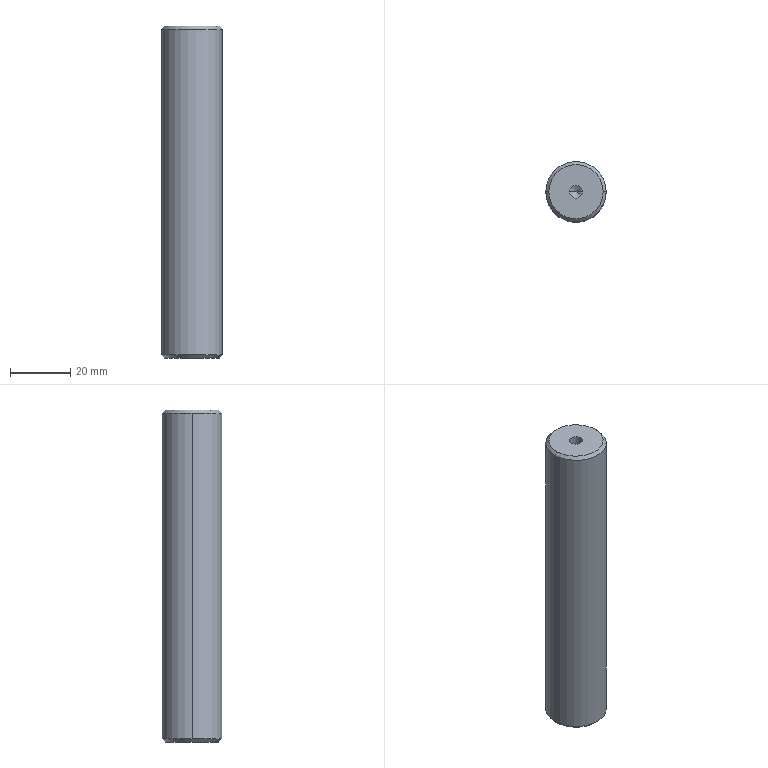Part | STEP file | 1 solid | 16 faces | box 20 x 20 x 110 mm | volume 33959 mm3 | cone 8 | cylinder 6 | plane 2 | commonest cylinder face diameters 4.2 x4 20 x2
STEP:
#1=CARTESIAN_POINT('',(0.,0.,0.));
#2=DIRECTION('',(0.,0.,1.));
#3=DIRECTION('',(1.,0.,0.));
#4=AXIS2_PLACEMENT_3D('',#1,#2,#3);
#5=CARTESIAN_POINT('',(9.,0.,110.));
#6=VERTEX_POINT('',#5);
#7=CARTESIAN_POINT('',(-9.,0.,110.));
#8=VERTEX_POINT('',#7);
#9=CARTESIAN_POINT('',(0.,0.,110.));
#10=DIRECTION('',(0.,0.,1.));
#11=DIRECTION('',(1.,0.,0.));
#12=AXIS2_PLACEMENT_3D('',#9,#10,#11);
#13=CIRCLE('',#12,9.);
#14=CARTESIAN_POINT('',(0.,0.,110.));
#15=DIRECTION('',(0.,0.,-1.));
#16=DIRECTION('',(-1.,0.,0.));
#17=AXIS2_PLACEMENT_3D('',#14,#15,#16);
#18=CONICAL_SURFACE('',#17,9.,0.7854);
#19=CARTESIAN_POINT('',(3.142,0.));
#20=DIRECTION('',(-1.,0.));
#21=VECTOR('',#20,1.);
#22=LINE('',#19,#21);
#23=(GEOMETRIC_REPRESENTATION_CONTEXT(2)PARAMETRIC_REPRESENTATION_CONTEXT()REPRESENTATION_CONTEXT('',''));
#24=DEFINITIONAL_REPRESENTATION('',(#22),#23);
#25=PCURVE('',#18,#24);
#26=CARTESIAN_POINT('',(0.,0.,110.));
#27=DIRECTION('',(0.,0.,1.));
#28=DIRECTION('',(1.,0.,0.));
#29=AXIS2_PLACEMENT_3D('',#26,#27,#28);
#30=PLANE('',#29);
#31=CARTESIAN_POINT('',(0.,0.));
#32=DIRECTION('',(1.,0.));
#33=AXIS2_PLACEMENT_2D('',#31,#32);
#34=CIRCLE('',#33,9.);
#35=(GEOMETRIC_REPRESENTATION_CONTEXT(2)PARAMETRIC_REPRESENTATION_CONTEXT()REPRESENTATION_CONTEXT('',''));
#36=DEFINITIONAL_REPRESENTATION('',(#34),#35);
#37=PCURVE('',#30,#36);
#38=SURFACE_CURVE('',#13,(#25,#37),.PCURVE_S1.);
#39=EDGE_CURVE('',#6,#8,#38,.T.);
#40=ORIENTED_EDGE('',*,*,#39,.F.);
#41=CARTESIAN_POINT('',(10.,0.,109.));
#42=VERTEX_POINT('',#41);
#43=CARTESIAN_POINT('',(9.,0.,110.));
#44=DIRECTION('',(0.7071,0.,-0.7071));
#45=VECTOR('',#44,1.);
#46=LINE('',#43,#45);
#47=CARTESIAN_POINT('',(3.142,0.));
#48=DIRECTION('',(0.,1.));
#49=VECTOR('',#48,1.);
#50=LINE('',#47,#49);
#51=(GEOMETRIC_REPRESENTATION_CONTEXT(2)PARAMETRIC_REPRESENTATION_CONTEXT()REPRESENTATION_CONTEXT('',''));
#52=DEFINITIONAL_REPRESENTATION('',(#50),#51);
#53=PCURVE('',#18,#52);
#54=CARTESIAN_POINT('',(0.,0.,110.));
#55=DIRECTION('',(0.,0.,-1.));
#56=DIRECTION('',(-1.,0.,0.));
#57=AXIS2_PLACEMENT_3D('',#54,#55,#56);
#58=CONICAL_SURFACE('',#57,9.,0.7854);
#59=CARTESIAN_POINT('',(3.142,0.));
#60=DIRECTION('',(0.,1.));
#61=VECTOR('',#60,1.);
#62=LINE('',#59,#61);
#63=(GEOMETRIC_REPRESENTATION_CONTEXT(2)PARAMETRIC_REPRESENTATION_CONTEXT()REPRESENTATION_CONTEXT('',''));
#64=DEFINITIONAL_REPRESENTATION('',(#62),#63);
#65=PCURVE('',#58,#64);
#66=SURFACE_CURVE('',#46,(#53,#65),.PCURVE_S1.);
#67=EDGE_CURVE('',#6,#42,#66,.T.);
#68=ORIENTED_EDGE('',*,*,#67,.T.);
#69=CARTESIAN_POINT('',(-10.,0.,109.));
#70=VERTEX_POINT('',#69);
#71=CARTESIAN_POINT('',(0.,0.,109.));
#72=DIRECTION('',(0.,0.,-1.));
#73=DIRECTION('',(1.,0.,0.));
#74=AXIS2_PLACEMENT_3D('',#71,#72,#73);
#75=CIRCLE('',#74,10.);
#76=CARTESIAN_POINT('',(-3.142,1.));
#77=DIRECTION('',(1.,0.));
#78=VECTOR('',#77,1.);
#79=LINE('',#76,#78);
#80=(GEOMETRIC_REPRESENTATION_CONTEXT(2)PARAMETRIC_REPRESENTATION_CONTEXT()REPRESENTATION_CONTEXT('',''));
#81=DEFINITIONAL_REPRESENTATION('',(#79),#80);
#82=PCURVE('',#18,#81);
#83=CARTESIAN_POINT('',(0.,0.,110.));
#84=DIRECTION('',(0.,0.,-1.));
#85=DIRECTION('',(-1.,0.,0.));
#86=AXIS2_PLACEMENT_3D('',#83,#84,#85);
#87=CYLINDRICAL_SURFACE('',#86,10.);
#88=CARTESIAN_POINT('',(-3.142,1.));
#89=DIRECTION('',(1.,0.));
#90=VECTOR('',#89,1.);
#91=LINE('',#88,#90);
#92=(GEOMETRIC_REPRESENTATION_CONTEXT(2)PARAMETRIC_REPRESENTATION_CONTEXT()REPRESENTATION_CONTEXT('',''));
#93=DEFINITIONAL_REPRESENTATION('',(#91),#92);
#94=PCURVE('',#87,#93);
#95=SURFACE_CURVE('',#75,(#82,#94),.PCURVE_S1.);
#96=EDGE_CURVE('',#70,#42,#95,.T.);
#97=ORIENTED_EDGE('',*,*,#96,.F.);
#98=CARTESIAN_POINT('',(-9.,0.,110.));
#99=DIRECTION('',(-0.7071,0.,-0.7071));
#100=VECTOR('',#99,1.);
#101=LINE('',#98,#100);
#102=CARTESIAN_POINT('',(0.,0.));
#103=DIRECTION('',(0.,1.));
#104=VECTOR('',#103,1.);
#105=LINE('',#102,#104);
#106=(GEOMETRIC_REPRESENTATION_CONTEXT(2)PARAMETRIC_REPRESENTATION_CONTEXT()REPRESENTATION_CONTEXT('',''));
#107=DEFINITIONAL_REPRESENTATION('',(#105),#106);
#108=PCURVE('',#18,#107);
#109=CARTESIAN_POINT('',(6.283,0.));
#110=DIRECTION('',(0.,1.));
#111=VECTOR('',#110,1.);
#112=LINE('',#109,#111);
#113=(GEOMETRIC_REPRESENTATION_CONTEXT(2)PARAMETRIC_REPRESENTATION_CONTEXT()REPRESENTATION_CONTEXT('',''));
#114=DEFINITIONAL_REPRESENTATION('',(#112),#113);
#115=PCURVE('',#58,#114);
#116=SURFACE_CURVE('',#101,(#108,#115),.PCURVE_S1.);
#117=EDGE_CURVE('',#8,#70,#116,.T.);
#118=ORIENTED_EDGE('',*,*,#117,.F.);
#119=EDGE_LOOP('',(#40,#68,#97,#118));
#120=FACE_BOUND('',#119,.T.);
#121=ADVANCED_FACE('',(#120),#18,.T.);
#122=CARTESIAN_POINT('',(-9.,0.,0.));
#123=VERTEX_POINT('',#122);
#124=CARTESIAN_POINT('',(9.,0.,0.));
#125=VERTEX_POINT('',#124);
#126=CARTESIAN_POINT('',(0.,0.,0.));
#127=DIRECTION('',(0.,0.,-1.));
#128=DIRECTION('',(1.,0.,0.));
#129=AXIS2_PLACEMENT_3D('',#126,#127,#128);
#130=CIRCLE('',#129,9.);
#131=CARTESIAN_POINT('',(0.,0.,1.));
#132=DIRECTION('',(0.,0.,1.));
#133=DIRECTION('',(1.,0.,0.));
#134=AXIS2_PLACEMENT_3D('',#131,#132,#133);
#135=CONICAL_SURFACE('',#134,10.,0.7854);
#136=CARTESIAN_POINT('',(6.283,-1.));
#137=DIRECTION('',(-1.,0.));
#138=VECTOR('',#137,1.);
#139=LINE('',#136,#138);
#140=(GEOMETRIC_REPRESENTATION_CONTEXT(2)PARAMETRIC_REPRESENTATION_CONTEXT()REPRESENTATION_CONTEXT('',''));
#141=DEFINITIONAL_REPRESENTATION('',(#139),#140);
#142=PCURVE('',#135,#141);
#143=CARTESIAN_POINT('',(0.,0.,0.));
#144=DIRECTION('',(0.,0.,1.));
#145=DIRECTION('',(1.,0.,0.));
#146=AXIS2_PLACEMENT_3D('',#143,#144,#145);
#147=PLANE('',#146);
#148=CARTESIAN_POINT('',(9.,0.));
#149=CARTESIAN_POINT('',(9.,-15.588));
#150=CARTESIAN_POINT('',(-4.5,-7.794));
#151=CARTESIAN_POINT('',(-18.,0.));
#152=CARTESIAN_POINT('',(-4.5,7.794));
#153=CARTESIAN_POINT('',(9.,15.588));
#154=CARTESIAN_POINT('',(9.,0.));
#155=(BOUNDED_CURVE()B_SPLINE_CURVE(2,(#148,#149,#150,#151,#152,#153,#154),.UNSPECIFIED.,.T.,.F.)B_SPLINE_CURVE_WITH_KNOTS((1,2,2,2,2,1),(-2.094,0.,2.094,4.189,6.283,8.378),.UNSPECIFIED.)CURVE()GEOMETRIC_REPRESENTATION_ITEM()RATIONAL_B_SPLINE_CURVE((1.,0.5,1.,0.5,1.,0.5,1.))REPRESENTATION_ITEM(''));
#156=(GEOMETRIC_REPRESENTATION_CONTEXT(2)PARAMETRIC_REPRESENTATION_CONTEXT()REPRESENTATION_CONTEXT('',''));
#157=DEFINITIONAL_REPRESENTATION('',(#155),#156);
#158=PCURVE('',#147,#157);
#159=SURFACE_CURVE('',#130,(#142,#158),.PCURVE_S1.);
#160=EDGE_CURVE('',#123,#125,#159,.T.);
#161=ORIENTED_EDGE('',*,*,#160,.F.);
#162=CARTESIAN_POINT('',(-10.,0.,1.));
#163=VERTEX_POINT('',#162);
#164=CARTESIAN_POINT('',(-10.,0.,1.));
#165=DIRECTION('',(-0.7071,0.,0.7071));
#166=VECTOR('',#165,1.);
#167=LINE('',#164,#166);
#168=CARTESIAN_POINT('',(3.142,0.));
#169=DIRECTION('',(0.,1.));
#170=VECTOR('',#169,1.);
#171=LINE('',#168,#170);
#172=(GEOMETRIC_REPRESENTATION_CONTEXT(2)PARAMETRIC_REPRESENTATION_CONTEXT()REPRESENTATION_CONTEXT('',''));
#173=DEFINITIONAL_REPRESENTATION('',(#171),#172);
#174=PCURVE('',#135,#173);
#175=CARTESIAN_POINT('',(0.,0.,1.));
#176=DIRECTION('',(0.,0.,1.));
#177=DIRECTION('',(1.,0.,0.));
#178=AXIS2_PLACEMENT_3D('',#175,#176,#177);
#179=CONICAL_SURFACE('',#178,10.,0.7854);
#180=CARTESIAN_POINT('',(3.142,0.));
#181=DIRECTION('',(0.,1.));
#182=VECTOR('',#181,1.);
#183=LINE('',#180,#182);
#184=(GEOMETRIC_REPRESENTATION_CONTEXT(2)PARAMETRIC_REPRESENTATION_CONTEXT()REPRESENTATION_CONTEXT('',''));
#185=DEFINITIONAL_REPRESENTATION('',(#183),#184);
#186=PCURVE('',#179,#185);
#187=SURFACE_CURVE('',#167,(#174,#186),.PCURVE_S1.);
#188=EDGE_CURVE('',#123,#163,#187,.T.);
#189=ORIENTED_EDGE('',*,*,#188,.T.);
#190=CARTESIAN_POINT('',(10.,0.,1.));
#191=VERTEX_POINT('',#190);
#192=CARTESIAN_POINT('',(0.,0.,1.));
#193=DIRECTION('',(0.,0.,1.));
#194=DIRECTION('',(1.,0.,0.));
#195=AXIS2_PLACEMENT_3D('',#192,#193,#194);
#196=CIRCLE('',#195,10.);
#197=CARTESIAN_POINT('',(0.,0.));
#198=DIRECTION('',(1.,0.));
#199=VECTOR('',#198,1.);
#200=LINE('',#197,#199);
#201=(GEOMETRIC_REPRESENTATION_CONTEXT(2)PARAMETRIC_REPRESENTATION_CONTEXT()REPRESENTATION_CONTEXT('',''));
#202=DEFINITIONAL_REPRESENTATION('',(#200),#201);
#203=PCURVE('',#135,#202);
#204=CARTESIAN_POINT('',(3.142,109.));
#205=DIRECTION('',(-1.,0.));
#206=VECTOR('',#205,1.);
#207=LINE('',#204,#206);
#208=(GEOMETRIC_REPRESENTATION_CONTEXT(2)PARAMETRIC_REPRESENTATION_CONTEXT()REPRESENTATION_CONTEXT('',''));
#209=DEFINITIONAL_REPRESENTATION('',(#207),#208);
#210=PCURVE('',#87,#209);
#211=SURFACE_CURVE('',#196,(#203,#210),.PCURVE_S1.);
#212=EDGE_CURVE('',#191,#163,#211,.T.);
#213=ORIENTED_EDGE('',*,*,#212,.F.);
#214=CARTESIAN_POINT('',(10.,0.,1.));
#215=DIRECTION('',(0.7071,0.,0.7071));
#216=VECTOR('',#215,1.);
#217=LINE('',#214,#216);
#218=CARTESIAN_POINT('',(0.,0.));
#219=DIRECTION('',(0.,1.));
#220=VECTOR('',#219,1.);
#221=LINE('',#218,#220);
#222=(GEOMETRIC_REPRESENTATION_CONTEXT(2)PARAMETRIC_REPRESENTATION_CONTEXT()REPRESENTATION_CONTEXT('',''));
#223=DEFINITIONAL_REPRESENTATION('',(#221),#222);
#224=PCURVE('',#135,#223);
#225=CARTESIAN_POINT('',(6.283,0.));
#226=DIRECTION('',(0.,1.));
#227=VECTOR('',#226,1.);
#228=LINE('',#225,#227);
#229=(GEOMETRIC_REPRESENTATION_CONTEXT(2)PARAMETRIC_REPRESENTATION_CONTEXT()REPRESENTATION_CONTEXT('',''));
#230=DEFINITIONAL_REPRESENTATION('',(#228),#229);
#231=PCURVE('',#179,#230);
#232=SURFACE_CURVE('',#217,(#224,#231),.PCURVE_S1.);
#233=EDGE_CURVE('',#125,#191,#232,.T.);
#234=ORIENTED_EDGE('',*,*,#233,.F.);
#235=EDGE_LOOP('',(#161,#189,#213,#234));
#236=FACE_BOUND('',#235,.T.);
#237=ADVANCED_FACE('',(#236),#135,.T.);
#238=CARTESIAN_POINT('',(2.1,0.,91.));
#239=VERTEX_POINT('',#238);
#240=CARTESIAN_POINT('',(2.1,0.,110.));
#241=VERTEX_POINT('',#240);
#242=CARTESIAN_POINT('',(2.1,0.,110.));
#243=DIRECTION('',(0.,0.,1.));
#244=VECTOR('',#243,1.);
#245=LINE('',#242,#244);
#246=CARTESIAN_POINT('',(0.,0.,110.));
#247=DIRECTION('',(0.,0.,1.));
#248=DIRECTION('',(1.,0.,0.));
#249=AXIS2_PLACEMENT_3D('',#246,#247,#248);
#250=CYLINDRICAL_SURFACE('',#249,2.1);
#251=CARTESIAN_POINT('',(6.283,0.));
#252=DIRECTION('',(0.,1.));
#253=VECTOR('',#252,1.);
#254=LINE('',#251,#253);
#255=(GEOMETRIC_REPRESENTATION_CONTEXT(2)PARAMETRIC_REPRESENTATION_CONTEXT()REPRESENTATION_CONTEXT('',''));
#256=DEFINITIONAL_REPRESENTATION('',(#254),#255);
#257=PCURVE('',#250,#256);
#258=CARTESIAN_POINT('',(0.,0.,110.));
#259=DIRECTION('',(0.,0.,1.));
#260=DIRECTION('',(1.,0.,0.));
#261=AXIS2_PLACEMENT_3D('',#258,#259,#260);
#262=CYLINDRICAL_SURFACE('',#261,2.1);
#263=CARTESIAN_POINT('',(0.,0.));
#264=DIRECTION('',(0.,1.));
#265=VECTOR('',#264,1.);
#266=LINE('',#263,#265);
#267=(GEOMETRIC_REPRESENTATION_CONTEXT(2)PARAMETRIC_REPRESENTATION_CONTEXT()REPRESENTATION_CONTEXT('',''));
#268=DEFINITIONAL_REPRESENTATION('',(#266),#267);
#269=PCURVE('',#262,#268);
#270=SURFACE_CURVE('',#245,(#257,#269),.PCURVE_S1.);
#271=EDGE_CURVE('',#239,#241,#270,.T.);
#272=ORIENTED_EDGE('',*,*,#271,.T.);
#273=CARTESIAN_POINT('',(-2.1,0.,110.));
#274=VERTEX_POINT('',#273);
#275=CARTESIAN_POINT('',(0.,0.,110.));
#276=DIRECTION('',(0.,0.,1.));
#277=DIRECTION('',(1.,0.,0.));
#278=AXIS2_PLACEMENT_3D('',#275,#276,#277);
#279=CIRCLE('',#278,2.1);
#280=CARTESIAN_POINT('',(0.,0.));
#281=DIRECTION('',(1.,0.));
#282=VECTOR('',#281,1.);
#283=LINE('',#280,#282);
#284=(GEOMETRIC_REPRESENTATION_CONTEXT(2)PARAMETRIC_REPRESENTATION_CONTEXT()REPRESENTATION_CONTEXT('',''));
#285=DEFINITIONAL_REPRESENTATION('',(#283),#284);
#286=PCURVE('',#250,#285);
#287=CARTESIAN_POINT('',(0.,0.));
#288=DIRECTION('',(1.,0.));
#289=AXIS2_PLACEMENT_2D('',#287,#288);
#290=CIRCLE('',#289,2.1);
#291=(GEOMETRIC_REPRESENTATION_CONTEXT(2)PARAMETRIC_REPRESENTATION_CONTEXT()REPRESENTATION_CONTEXT('',''));
#292=DEFINITIONAL_REPRESENTATION('',(#290),#291);
#293=PCURVE('',#30,#292);
#294=SURFACE_CURVE('',#279,(#286,#293),.PCURVE_S1.);
#295=EDGE_CURVE('',#274,#241,#294,.T.);
#296=ORIENTED_EDGE('',*,*,#295,.F.);
#297=CARTESIAN_POINT('',(-2.1,0.,91.));
#298=VERTEX_POINT('',#297);
#299=CARTESIAN_POINT('',(-2.1,0.,110.));
#300=DIRECTION('',(0.,0.,1.));
#301=VECTOR('',#300,1.);
#302=LINE('',#299,#301);
#303=CARTESIAN_POINT('',(3.142,0.));
#304=DIRECTION('',(0.,1.));
#305=VECTOR('',#304,1.);
#306=LINE('',#303,#305);
#307=(GEOMETRIC_REPRESENTATION_CONTEXT(2)PARAMETRIC_REPRESENTATION_CONTEXT()REPRESENTATION_CONTEXT('',''));
#308=DEFINITIONAL_REPRESENTATION('',(#306),#307);
#309=PCURVE('',#250,#308);
#310=CARTESIAN_POINT('',(3.142,0.));
#311=DIRECTION('',(0.,1.));
#312=VECTOR('',#311,1.);
#313=LINE('',#310,#312);
#314=(GEOMETRIC_REPRESENTATION_CONTEXT(2)PARAMETRIC_REPRESENTATION_CONTEXT()REPRESENTATION_CONTEXT('',''));
#315=DEFINITIONAL_REPRESENTATION('',(#313),#314);
#316=PCURVE('',#262,#315);
#317=SURFACE_CURVE('',#302,(#309,#316),.PCURVE_S1.);
#318=EDGE_CURVE('',#298,#274,#317,.T.);
#319=ORIENTED_EDGE('',*,*,#318,.F.);
#320=CARTESIAN_POINT('',(0.,0.,91.));
#321=DIRECTION('',(0.,0.,1.));
#322=DIRECTION('',(1.,0.,0.));
#323=AXIS2_PLACEMENT_3D('',#320,#321,#322);
#324=CIRCLE('',#323,2.1);
#325=CARTESIAN_POINT('',(0.,-19.));
#326=DIRECTION('',(1.,0.));
#327=VECTOR('',#326,1.);
#328=LINE('',#325,#327);
#329=(GEOMETRIC_REPRESENTATION_CONTEXT(2)PARAMETRIC_REPRESENTATION_CONTEXT()REPRESENTATION_CONTEXT('',''));
#330=DEFINITIONAL_REPRESENTATION('',(#328),#329);
#331=PCURVE('',#250,#330);
#332=CARTESIAN_POINT('',(0.,0.,91.));
#333=DIRECTION('',(0.,0.,1.));
#334=DIRECTION('',(1.,0.,0.));
#335=AXIS2_PLACEMENT_3D('',#332,#333,#334);
#336=CONICAL_SURFACE('',#335,2.1,1.03);
#337=CARTESIAN_POINT('',(0.,0.));
#338=DIRECTION('',(1.,0.));
#339=VECTOR('',#338,1.);
#340=LINE('',#337,#339);
#341=(GEOMETRIC_REPRESENTATION_CONTEXT(2)PARAMETRIC_REPRESENTATION_CONTEXT()REPRESENTATION_CONTEXT('',''));
#342=DEFINITIONAL_REPRESENTATION('',(#340),#341);
#343=PCURVE('',#336,#342);
#344=SURFACE_CURVE('',#324,(#331,#343),.PCURVE_S1.);
#345=EDGE_CURVE('',#298,#239,#344,.T.);
#346=ORIENTED_EDGE('',*,*,#345,.T.);
#347=EDGE_LOOP('',(#272,#296,#319,#346));
#348=FACE_BOUND('',#347,.F.);
#349=ADVANCED_FACE('',(#348),#250,.F.);
#350=ORIENTED_EDGE('',*,*,#345,.F.);
#351=CARTESIAN_POINT('',(0.,0.,89.738));
#352=VERTEX_POINT('',#351);
#353=CARTESIAN_POINT('',(-2.1,0.,91.));
#354=DIRECTION('',(-0.8572,0.,0.515));
#355=VECTOR('',#354,1.);
#356=LINE('',#353,#355);
#357=CARTESIAN_POINT('',(3.142,0.));
#358=DIRECTION('',(0.,1.));
#359=VECTOR('',#358,1.);
#360=LINE('',#357,#359);
#361=(GEOMETRIC_REPRESENTATION_CONTEXT(2)PARAMETRIC_REPRESENTATION_CONTEXT()REPRESENTATION_CONTEXT('',''));
#362=DEFINITIONAL_REPRESENTATION('',(#360),#361);
#363=PCURVE('',#336,#362);
#364=CARTESIAN_POINT('',(0.,0.,91.));
#365=DIRECTION('',(0.,0.,1.));
#366=DIRECTION('',(1.,0.,0.));
#367=AXIS2_PLACEMENT_3D('',#364,#365,#366);
#368=CONICAL_SURFACE('',#367,2.1,1.03);
#369=CARTESIAN_POINT('',(3.142,0.));
#370=DIRECTION('',(0.,1.));
#371=VECTOR('',#370,1.);
#372=LINE('',#369,#371);
#373=(GEOMETRIC_REPRESENTATION_CONTEXT(2)PARAMETRIC_REPRESENTATION_CONTEXT()REPRESENTATION_CONTEXT('',''));
#374=DEFINITIONAL_REPRESENTATION('',(#372),#373);
#375=PCURVE('',#368,#374);
#376=SURFACE_CURVE('',#356,(#363,#375),.PCURVE_S1.);
#377=EDGE_CURVE('',#352,#298,#376,.T.);
#378=ORIENTED_EDGE('',*,*,#377,.F.);
#379=CARTESIAN_POINT('',(2.1,0.,91.));
#380=DIRECTION('',(0.8572,0.,0.515));
#381=VECTOR('',#380,1.);
#382=LINE('',#379,#381);
#383=CARTESIAN_POINT('',(6.283,-1.262));
#384=CARTESIAN_POINT('',(6.283,-1.243));
#385=CARTESIAN_POINT('',(6.283,-1.204));
#386=CARTESIAN_POINT('',(6.283,-1.147));
#387=CARTESIAN_POINT('',(6.283,-1.09));
#388=CARTESIAN_POINT('',(6.283,-1.032));
#389=CARTESIAN_POINT('',(6.283,-0.975));
#390=CARTESIAN_POINT('',(6.283,-0.9177));
#391=CARTESIAN_POINT('',(6.283,-0.8603));
#392=CARTESIAN_POINT('',(6.283,-0.803));
#393=CARTESIAN_POINT('',(6.283,-0.7456));
#394=CARTESIAN_POINT('',(6.283,-0.6883));
#395=CARTESIAN_POINT('',(6.283,-0.6309));
#396=CARTESIAN_POINT('',(6.283,-0.5735));
#397=CARTESIAN_POINT('',(6.283,-0.5162));
#398=CARTESIAN_POINT('',(6.283,-0.4588));
#399=CARTESIAN_POINT('',(6.283,-0.4015));
#400=CARTESIAN_POINT('',(6.283,-0.3441));
#401=CARTESIAN_POINT('',(6.283,-0.2868));
#402=CARTESIAN_POINT('',(6.283,-0.2294));
#403=CARTESIAN_POINT('',(6.283,-0.1721));
#404=CARTESIAN_POINT('',(6.283,-0.1147));
#405=CARTESIAN_POINT('',(6.283,-0.05735));
#406=CARTESIAN_POINT('',(6.283,-0.01912));
#407=CARTESIAN_POINT('',(6.283,0.));
#408=B_SPLINE_CURVE_WITH_KNOTS('',3,(#383,#384,#385,#386,#387,#388,#389,#390,#391,#392,#393,#394,#395,#396,#397,#398,#399,#400,#401,#402,#403,#404,#405,#406,#407),.UNSPECIFIED.,.F.,.F.,(4,1,1,1,1,1,1,1,1,1,1,1,1,1,1,1,1,1,1,1,1,1,4),(-2.45,-2.339,-2.227,-2.116,-2.004,-1.893,-1.782,-1.67,-1.559,-1.448,-1.336,-1.225,-1.114,-1.002,-0.8909,-0.7795,-0.6682,-0.5568,-0.4454,-0.3341,-0.2227,-0.1114,0.),.QUASI_UNIFORM_KNOTS.);
#409=(GEOMETRIC_REPRESENTATION_CONTEXT(2)PARAMETRIC_REPRESENTATION_CONTEXT()REPRESENTATION_CONTEXT('',''));
#410=DEFINITIONAL_REPRESENTATION('',(#408),#409);
#411=PCURVE('',#336,#410);
#412=CARTESIAN_POINT('',(0.,-1.262));
#413=CARTESIAN_POINT('',(0.,-1.243));
#414=CARTESIAN_POINT('',(0.,-1.204));
#415=CARTESIAN_POINT('',(0.,-1.147));
#416=CARTESIAN_POINT('',(0.,-1.09));
#417=CARTESIAN_POINT('',(0.,-1.032));
#418=CARTESIAN_POINT('',(0.,-0.975));
#419=CARTESIAN_POINT('',(0.,-0.9177));
#420=CARTESIAN_POINT('',(0.,-0.8603));
#421=CARTESIAN_POINT('',(0.,-0.803));
#422=CARTESIAN_POINT('',(0.,-0.7456));
#423=CARTESIAN_POINT('',(0.,-0.6883));
#424=CARTESIAN_POINT('',(0.,-0.6309));
#425=CARTESIAN_POINT('',(0.,-0.5735));
#426=CARTESIAN_POINT('',(0.,-0.5162));
#427=CARTESIAN_POINT('',(0.,-0.4588));
#428=CARTESIAN_POINT('',(0.,-0.4015));
#429=CARTESIAN_POINT('',(0.,-0.3441));
#430=CARTESIAN_POINT('',(0.,-0.2868));
#431=CARTESIAN_POINT('',(0.,-0.2294));
#432=CARTESIAN_POINT('',(0.,-0.1721));
#433=CARTESIAN_POINT('',(0.,-0.1147));
#434=CARTESIAN_POINT('',(0.,-0.05735));
#435=CARTESIAN_POINT('',(0.,-0.01912));
#436=CARTESIAN_POINT('',(0.,0.));
#437=B_SPLINE_CURVE_WITH_KNOTS('',3,(#412,#413,#414,#415,#416,#417,#418,#419,#420,#421,#422,#423,#424,#425,#426,#427,#428,#429,#430,#431,#432,#433,#434,#435,#436),.UNSPECIFIED.,.F.,.F.,(4,1,1,1,1,1,1,1,1,1,1,1,1,1,1,1,1,1,1,1,1,1,4),(-2.45,-2.339,-2.227,-2.116,-2.004,-1.893,-1.782,-1.67,-1.559,-1.448,-1.336,-1.225,-1.114,-1.002,-0.8909,-0.7795,-0.6682,-0.5568,-0.4454,-0.3341,-0.2227,-0.1114,0.),.QUASI_UNIFORM_KNOTS.);
#438=(GEOMETRIC_REPRESENTATION_CONTEXT(2)PARAMETRIC_REPRESENTATION_CONTEXT()REPRESENTATION_CONTEXT('',''));
#439=DEFINITIONAL_REPRESENTATION('',(#437),#438);
#440=PCURVE('',#368,#439);
#441=SURFACE_CURVE('',#382,(#411,#440),.PCURVE_S1.);
#442=EDGE_CURVE('',#352,#239,#441,.T.);
#443=ORIENTED_EDGE('',*,*,#442,.T.);
#444=EDGE_LOOP('',(#350,#378,#443));
#445=FACE_BOUND('',#444,.F.);
#446=ADVANCED_FACE('',(#445),#336,.F.);
#447=CARTESIAN_POINT('',(-2.1,0.,19.));
#448=VERTEX_POINT('',#447);
#449=CARTESIAN_POINT('',(-2.1,0.,0.));
#450=VERTEX_POINT('',#449);
#451=CARTESIAN_POINT('',(-2.1,0.,0.));
#452=DIRECTION('',(0.,0.,-1.));
#453=VECTOR('',#452,1.);
#454=LINE('',#451,#453);
#455=CARTESIAN_POINT('',(0.,0.,0.));
#456=DIRECTION('',(0.,0.,-1.));
#457=DIRECTION('',(-1.,0.,0.));
#458=AXIS2_PLACEMENT_3D('',#455,#456,#457);
#459=CYLINDRICAL_SURFACE('',#458,2.1);
#460=CARTESIAN_POINT('',(6.283,0.));
#461=DIRECTION('',(0.,1.));
#462=VECTOR('',#461,1.);
#463=LINE('',#460,#462);
#464=(GEOMETRIC_REPRESENTATION_CONTEXT(2)PARAMETRIC_REPRESENTATION_CONTEXT()REPRESENTATION_CONTEXT('',''));
#465=DEFINITIONAL_REPRESENTATION('',(#463),#464);
#466=PCURVE('',#459,#465);
#467=CARTESIAN_POINT('',(0.,0.,0.));
#468=DIRECTION('',(0.,0.,-1.));
#469=DIRECTION('',(-1.,0.,0.));
#470=AXIS2_PLACEMENT_3D('',#467,#468,#469);
#471=CYLINDRICAL_SURFACE('',#470,2.1);
#472=CARTESIAN_POINT('',(0.,0.));
#473=DIRECTION('',(0.,1.));
#474=VECTOR('',#473,1.);
#475=LINE('',#472,#474);
#476=(GEOMETRIC_REPRESENTATION_CONTEXT(2)PARAMETRIC_REPRESENTATION_CONTEXT()REPRESENTATION_CONTEXT('',''));
#477=DEFINITIONAL_REPRESENTATION('',(#475),#476);
#478=PCURVE('',#471,#477);
#479=SURFACE_CURVE('',#454,(#466,#478),.PCURVE_S1.);
#480=EDGE_CURVE('',#448,#450,#479,.T.);
#481=ORIENTED_EDGE('',*,*,#480,.T.);
#482=CARTESIAN_POINT('',(2.1,0.,0.));
#483=VERTEX_POINT('',#482);
#484=CARTESIAN_POINT('',(0.,0.,0.));
#485=DIRECTION('',(0.,0.,-1.));
#486=DIRECTION('',(-1.,0.,0.));
#487=AXIS2_PLACEMENT_3D('',#484,#485,#486);
#488=CIRCLE('',#487,2.1);
#489=CARTESIAN_POINT('',(0.,0.));
#490=DIRECTION('',(1.,0.));
#491=VECTOR('',#490,1.);
#492=LINE('',#489,#491);
#493=(GEOMETRIC_REPRESENTATION_CONTEXT(2)PARAMETRIC_REPRESENTATION_CONTEXT()REPRESENTATION_CONTEXT('',''));
#494=DEFINITIONAL_REPRESENTATION('',(#492),#493);
#495=PCURVE('',#459,#494);
#496=CARTESIAN_POINT('',(-2.1,0.));
#497=CARTESIAN_POINT('',(-2.1,3.637));
#498=CARTESIAN_POINT('',(1.05,1.819));
#499=CARTESIAN_POINT('',(4.2,0.));
#500=CARTESIAN_POINT('',(1.05,-1.819));
#501=CARTESIAN_POINT('',(-2.1,-3.637));
#502=CARTESIAN_POINT('',(-2.1,0.));
#503=(BOUNDED_CURVE()B_SPLINE_CURVE(2,(#496,#497,#498,#499,#500,#501,#502),.UNSPECIFIED.,.T.,.F.)B_SPLINE_CURVE_WITH_KNOTS((1,2,2,2,2,1),(-2.094,0.,2.094,4.189,6.283,8.378),.UNSPECIFIED.)CURVE()GEOMETRIC_REPRESENTATION_ITEM()RATIONAL_B_SPLINE_CURVE((1.,0.5,1.,0.5,1.,0.5,1.))REPRESENTATION_ITEM(''));
#504=(GEOMETRIC_REPRESENTATION_CONTEXT(2)PARAMETRIC_REPRESENTATION_CONTEXT()REPRESENTATION_CONTEXT('',''));
#505=DEFINITIONAL_REPRESENTATION('',(#503),#504);
#506=PCURVE('',#147,#505);
#507=SURFACE_CURVE('',#488,(#495,#506),.PCURVE_S1.);
#508=EDGE_CURVE('',#483,#450,#507,.T.);
#509=ORIENTED_EDGE('',*,*,#508,.F.);
#510=CARTESIAN_POINT('',(2.1,0.,19.));
#511=VERTEX_POINT('',#510);
#512=CARTESIAN_POINT('',(2.1,0.,0.));
#513=DIRECTION('',(0.,0.,-1.));
#514=VECTOR('',#513,1.);
#515=LINE('',#512,#514);
#516=CARTESIAN_POINT('',(3.142,0.));
#517=DIRECTION('',(0.,1.));
#518=VECTOR('',#517,1.);
#519=LINE('',#516,#518);
#520=(GEOMETRIC_REPRESENTATION_CONTEXT(2)PARAMETRIC_REPRESENTATION_CONTEXT()REPRESENTATION_CONTEXT('',''));
#521=DEFINITIONAL_REPRESENTATION('',(#519),#520);
#522=PCURVE('',#459,#521);
#523=CARTESIAN_POINT('',(3.142,0.));
#524=DIRECTION('',(0.,1.));
#525=VECTOR('',#524,1.);
#526=LINE('',#523,#525);
#527=(GEOMETRIC_REPRESENTATION_CONTEXT(2)PARAMETRIC_REPRESENTATION_CONTEXT()REPRESENTATION_CONTEXT('',''));
#528=DEFINITIONAL_REPRESENTATION('',(#526),#527);
#529=PCURVE('',#471,#528);
#530=SURFACE_CURVE('',#515,(#522,#529),.PCURVE_S1.);
#531=EDGE_CURVE('',#511,#483,#530,.T.);
#532=ORIENTED_EDGE('',*,*,#531,.F.);
#533=CARTESIAN_POINT('',(0.,0.,19.));
#534=DIRECTION('',(0.,0.,-1.));
#535=DIRECTION('',(-1.,0.,0.));
#536=AXIS2_PLACEMENT_3D('',#533,#534,#535);
#537=CIRCLE('',#536,2.1);
#538=CARTESIAN_POINT('',(0.,-19.));
#539=DIRECTION('',(1.,0.));
#540=VECTOR('',#539,1.);
#541=LINE('',#538,#540);
#542=(GEOMETRIC_REPRESENTATION_CONTEXT(2)PARAMETRIC_REPRESENTATION_CONTEXT()REPRESENTATION_CONTEXT('',''));
#543=DEFINITIONAL_REPRESENTATION('',(#541),#542);
#544=PCURVE('',#459,#543);
#545=CARTESIAN_POINT('',(0.,0.,19.));
#546=DIRECTION('',(0.,0.,-1.));
#547=DIRECTION('',(-1.,0.,0.));
#548=AXIS2_PLACEMENT_3D('',#545,#546,#547);
#549=CONICAL_SURFACE('',#548,2.1,1.03);
#550=CARTESIAN_POINT('',(0.,0.));
#551=DIRECTION('',(1.,0.));
#552=VECTOR('',#551,1.);
#553=LINE('',#550,#552);
#554=(GEOMETRIC_REPRESENTATION_CONTEXT(2)PARAMETRIC_REPRESENTATION_CONTEXT()REPRESENTATION_CONTEXT('',''));
#555=DEFINITIONAL_REPRESENTATION('',(#553),#554);
#556=PCURVE('',#549,#555);
#557=SURFACE_CURVE('',#537,(#544,#556),.PCURVE_S1.);
#558=EDGE_CURVE('',#511,#448,#557,.T.);
#559=ORIENTED_EDGE('',*,*,#558,.T.);
#560=EDGE_LOOP('',(#481,#509,#532,#559));
#561=FACE_BOUND('',#560,.F.);
#562=ADVANCED_FACE('',(#561),#459,.F.);
#563=ORIENTED_EDGE('',*,*,#558,.F.);
#564=CARTESIAN_POINT('',(0.,0.,20.262));
#565=VERTEX_POINT('',#564);
#566=CARTESIAN_POINT('',(2.1,0.,19.));
#567=DIRECTION('',(0.8572,0.,-0.515));
#568=VECTOR('',#567,1.);
#569=LINE('',#566,#568);
#570=CARTESIAN_POINT('',(3.142,-1.262));
#571=CARTESIAN_POINT('',(3.142,-1.243));
#572=CARTESIAN_POINT('',(3.142,-1.204));
#573=CARTESIAN_POINT('',(3.142,-1.147));
#574=CARTESIAN_POINT('',(3.142,-1.09));
#575=CARTESIAN_POINT('',(3.142,-1.032));
#576=CARTESIAN_POINT('',(3.142,-0.975));
#577=CARTESIAN_POINT('',(3.142,-0.9177));
#578=CARTESIAN_POINT('',(3.142,-0.8603));
#579=CARTESIAN_POINT('',(3.142,-0.803));
#580=CARTESIAN_POINT('',(3.142,-0.7456));
#581=CARTESIAN_POINT('',(3.142,-0.6883));
#582=CARTESIAN_POINT('',(3.142,-0.6309));
#583=CARTESIAN_POINT('',(3.142,-0.5735));
#584=CARTESIAN_POINT('',(3.142,-0.5162));
#585=CARTESIAN_POINT('',(3.142,-0.4588));
#586=CARTESIAN_POINT('',(3.142,-0.4015));
#587=CARTESIAN_POINT('',(3.142,-0.3441));
#588=CARTESIAN_POINT('',(3.142,-0.2868));
#589=CARTESIAN_POINT('',(3.142,-0.2294));
#590=CARTESIAN_POINT('',(3.142,-0.1721));
#591=CARTESIAN_POINT('',(3.142,-0.1147));
#592=CARTESIAN_POINT('',(3.142,-0.05735));
#593=CARTESIAN_POINT('',(3.142,-0.01912));
#594=CARTESIAN_POINT('',(3.142,0.));
#595=B_SPLINE_CURVE_WITH_KNOTS('',3,(#570,#571,#572,#573,#574,#575,#576,#577,#578,#579,#580,#581,#582,#583,#584,#585,#586,#587,#588,#589,#590,#591,#592,#593,#594),.UNSPECIFIED.,.F.,.F.,(4,1,1,1,1,1,1,1,1,1,1,1,1,1,1,1,1,1,1,1,1,1,4),(-2.45,-2.339,-2.227,-2.116,-2.004,-1.893,-1.782,-1.67,-1.559,-1.448,-1.336,-1.225,-1.114,-1.002,-0.8909,-0.7795,-0.6682,-0.5568,-0.4454,-0.3341,-0.2227,-0.1114,0.),.UNSPECIFIED.);
#596=(GEOMETRIC_REPRESENTATION_CONTEXT(2)PARAMETRIC_REPRESENTATION_CONTEXT()REPRESENTATION_CONTEXT('',''));
#597=DEFINITIONAL_REPRESENTATION('',(#595),#596);
#598=PCURVE('',#549,#597);
#599=CARTESIAN_POINT('',(0.,0.,19.));
#600=DIRECTION('',(0.,0.,-1.));
#601=DIRECTION('',(-1.,0.,0.));
#602=AXIS2_PLACEMENT_3D('',#599,#600,#601);
#603=CONICAL_SURFACE('',#602,2.1,1.03);
#604=CARTESIAN_POINT('',(3.142,-1.262));
#605=CARTESIAN_POINT('',(3.142,-1.243));
#606=CARTESIAN_POINT('',(3.142,-1.204));
#607=CARTESIAN_POINT('',(3.142,-1.147));
#608=CARTESIAN_POINT('',(3.142,-1.09));
#609=CARTESIAN_POINT('',(3.142,-1.032));
#610=CARTESIAN_POINT('',(3.142,-0.975));
#611=CARTESIAN_POINT('',(3.142,-0.9177));
#612=CARTESIAN_POINT('',(3.142,-0.8603));
#613=CARTESIAN_POINT('',(3.142,-0.803));
#614=CARTESIAN_POINT('',(3.142,-0.7456));
#615=CARTESIAN_POINT('',(3.142,-0.6883));
#616=CARTESIAN_POINT('',(3.142,-0.6309));
#617=CARTESIAN_POINT('',(3.142,-0.5735));
#618=CARTESIAN_POINT('',(3.142,-0.5162));
#619=CARTESIAN_POINT('',(3.142,-0.4588));
#620=CARTESIAN_POINT('',(3.142,-0.4015));
#621=CARTESIAN_POINT('',(3.142,-0.3441));
#622=CARTESIAN_POINT('',(3.142,-0.2868));
#623=CARTESIAN_POINT('',(3.142,-0.2294));
#624=CARTESIAN_POINT('',(3.142,-0.1721));
#625=CARTESIAN_POINT('',(3.142,-0.1147));
#626=CARTESIAN_POINT('',(3.142,-0.05735));
#627=CARTESIAN_POINT('',(3.142,-0.01912));
#628=CARTESIAN_POINT('',(3.142,0.));
#629=B_SPLINE_CURVE_WITH_KNOTS('',3,(#604,#605,#606,#607,#608,#609,#610,#611,#612,#613,#614,#615,#616,#617,#618,#619,#620,#621,#622,#623,#624,#625,#626,#627,#628),.UNSPECIFIED.,.F.,.F.,(4,1,1,1,1,1,1,1,1,1,1,1,1,1,1,1,1,1,1,1,1,1,4),(-2.45,-2.339,-2.227,-2.116,-2.004,-1.893,-1.782,-1.67,-1.559,-1.448,-1.336,-1.225,-1.114,-1.002,-0.8909,-0.7795,-0.6682,-0.5568,-0.4454,-0.3341,-0.2227,-0.1114,0.),.UNSPECIFIED.);
#630=(GEOMETRIC_REPRESENTATION_CONTEXT(2)PARAMETRIC_REPRESENTATION_CONTEXT()REPRESENTATION_CONTEXT('',''));
#631=DEFINITIONAL_REPRESENTATION('',(#629),#630);
#632=PCURVE('',#603,#631);
#633=SURFACE_CURVE('',#569,(#598,#632),.PCURVE_S1.);
#634=EDGE_CURVE('',#565,#511,#633,.T.);
#635=ORIENTED_EDGE('',*,*,#634,.F.);
#636=CARTESIAN_POINT('',(-2.1,0.,19.));
#637=DIRECTION('',(-0.8572,0.,-0.515));
#638=VECTOR('',#637,1.);
#639=LINE('',#636,#638);
#640=CARTESIAN_POINT('',(6.283,0.));
#641=DIRECTION('',(0.,1.));
#642=VECTOR('',#641,1.);
#643=LINE('',#640,#642);
#644=(GEOMETRIC_REPRESENTATION_CONTEXT(2)PARAMETRIC_REPRESENTATION_CONTEXT()REPRESENTATION_CONTEXT('',''));
#645=DEFINITIONAL_REPRESENTATION('',(#643),#644);
#646=PCURVE('',#549,#645);
#647=CARTESIAN_POINT('',(0.,0.));
#648=DIRECTION('',(0.,1.));
#649=VECTOR('',#648,1.);
#650=LINE('',#647,#649);
#651=(GEOMETRIC_REPRESENTATION_CONTEXT(2)PARAMETRIC_REPRESENTATION_CONTEXT()REPRESENTATION_CONTEXT('',''));
#652=DEFINITIONAL_REPRESENTATION('',(#650),#651);
#653=PCURVE('',#603,#652);
#654=SURFACE_CURVE('',#639,(#646,#653),.PCURVE_S1.);
#655=EDGE_CURVE('',#565,#448,#654,.T.);
#656=ORIENTED_EDGE('',*,*,#655,.T.);
#657=EDGE_LOOP('',(#563,#635,#656));
#658=FACE_BOUND('',#657,.F.);
#659=ADVANCED_FACE('',(#658),#549,.F.);
#660=ORIENTED_EDGE('',*,*,#96,.T.);
#661=CARTESIAN_POINT('',(10.,0.,110.));
#662=DIRECTION('',(0.,0.,-1.));
#663=VECTOR('',#662,1.);
#664=LINE('',#661,#663);
#665=CARTESIAN_POINT('',(3.142,0.));
#666=DIRECTION('',(0.,1.));
#667=VECTOR('',#666,1.);
#668=LINE('',#665,#667);
#669=(GEOMETRIC_REPRESENTATION_CONTEXT(2)PARAMETRIC_REPRESENTATION_CONTEXT()REPRESENTATION_CONTEXT('',''));
#670=DEFINITIONAL_REPRESENTATION('',(#668),#669);
#671=PCURVE('',#87,#670);
#672=CARTESIAN_POINT('',(0.,0.,110.));
#673=DIRECTION('',(0.,0.,-1.));
#674=DIRECTION('',(-1.,0.,0.));
#675=AXIS2_PLACEMENT_3D('',#672,#673,#674);
#676=CYLINDRICAL_SURFACE('',#675,10.);
#677=CARTESIAN_POINT('',(3.142,0.));
#678=DIRECTION('',(0.,1.));
#679=VECTOR('',#678,1.);
#680=LINE('',#677,#679);
#681=(GEOMETRIC_REPRESENTATION_CONTEXT(2)PARAMETRIC_REPRESENTATION_CONTEXT()REPRESENTATION_CONTEXT('',''));
#682=DEFINITIONAL_REPRESENTATION('',(#680),#681);
#683=PCURVE('',#676,#682);
#684=SURFACE_CURVE('',#664,(#671,#683),.PCURVE_S1.);
#685=EDGE_CURVE('',#42,#191,#684,.T.);
#686=ORIENTED_EDGE('',*,*,#685,.T.);
#687=ORIENTED_EDGE('',*,*,#212,.T.);
#688=CARTESIAN_POINT('',(-10.,0.,110.));
#689=DIRECTION('',(0.,0.,-1.));
#690=VECTOR('',#689,1.);
#691=LINE('',#688,#690);
#692=CARTESIAN_POINT('',(0.,0.));
#693=DIRECTION('',(0.,1.));
#694=VECTOR('',#693,1.);
#695=LINE('',#692,#694);
#696=(GEOMETRIC_REPRESENTATION_CONTEXT(2)PARAMETRIC_REPRESENTATION_CONTEXT()REPRESENTATION_CONTEXT('',''));
#697=DEFINITIONAL_REPRESENTATION('',(#695),#696);
#698=PCURVE('',#87,#697);
#699=CARTESIAN_POINT('',(6.283,0.));
#700=DIRECTION('',(0.,1.));
#701=VECTOR('',#700,1.);
#702=LINE('',#699,#701);
#703=(GEOMETRIC_REPRESENTATION_CONTEXT(2)PARAMETRIC_REPRESENTATION_CONTEXT()REPRESENTATION_CONTEXT('',''));
#704=DEFINITIONAL_REPRESENTATION('',(#702),#703);
#705=PCURVE('',#676,#704);
#706=SURFACE_CURVE('',#691,(#698,#705),.PCURVE_S1.);
#707=EDGE_CURVE('',#70,#163,#706,.T.);
#708=ORIENTED_EDGE('',*,*,#707,.F.);
#709=EDGE_LOOP('',(#660,#686,#687,#708));
#710=FACE_BOUND('',#709,.T.);
#711=ADVANCED_FACE('',(#710),#87,.T.);
#712=ORIENTED_EDGE('',*,*,#685,.F.);
#713=CARTESIAN_POINT('',(0.,0.,109.));
#714=DIRECTION('',(0.,0.,-1.));
#715=DIRECTION('',(1.,0.,0.));
#716=AXIS2_PLACEMENT_3D('',#713,#714,#715);
#717=CIRCLE('',#716,10.);
#718=CARTESIAN_POINT('',(3.142,1.));
#719=DIRECTION('',(1.,0.));
#720=VECTOR('',#719,1.);
#721=LINE('',#718,#720);
#722=(GEOMETRIC_REPRESENTATION_CONTEXT(2)PARAMETRIC_REPRESENTATION_CONTEXT()REPRESENTATION_CONTEXT('',''));
#723=DEFINITIONAL_REPRESENTATION('',(#721),#722);
#724=PCURVE('',#676,#723);
#725=CARTESIAN_POINT('',(3.142,1.));
#726=DIRECTION('',(1.,0.));
#727=VECTOR('',#726,1.);
#728=LINE('',#725,#727);
#729=(GEOMETRIC_REPRESENTATION_CONTEXT(2)PARAMETRIC_REPRESENTATION_CONTEXT()REPRESENTATION_CONTEXT('',''));
#730=DEFINITIONAL_REPRESENTATION('',(#728),#729);
#731=PCURVE('',#58,#730);
#732=SURFACE_CURVE('',#717,(#724,#731),.PCURVE_S1.);
#733=EDGE_CURVE('',#42,#70,#732,.T.);
#734=ORIENTED_EDGE('',*,*,#733,.T.);
#735=ORIENTED_EDGE('',*,*,#707,.T.);
#736=CARTESIAN_POINT('',(0.,0.,1.));
#737=DIRECTION('',(0.,0.,1.));
#738=DIRECTION('',(1.,0.,0.));
#739=AXIS2_PLACEMENT_3D('',#736,#737,#738);
#740=CIRCLE('',#739,10.);
#741=CARTESIAN_POINT('',(9.425,109.));
#742=DIRECTION('',(-1.,0.));
#743=VECTOR('',#742,1.);
#744=LINE('',#741,#743);
#745=(GEOMETRIC_REPRESENTATION_CONTEXT(2)PARAMETRIC_REPRESENTATION_CONTEXT()REPRESENTATION_CONTEXT('',''));
#746=DEFINITIONAL_REPRESENTATION('',(#744),#745);
#747=PCURVE('',#676,#746);
#748=CARTESIAN_POINT('',(0.,0.));
#749=DIRECTION('',(1.,0.));
#750=VECTOR('',#749,1.);
#751=LINE('',#748,#750);
#752=(GEOMETRIC_REPRESENTATION_CONTEXT(2)PARAMETRIC_REPRESENTATION_CONTEXT()REPRESENTATION_CONTEXT('',''));
#753=DEFINITIONAL_REPRESENTATION('',(#751),#752);
#754=PCURVE('',#179,#753);
#755=SURFACE_CURVE('',#740,(#747,#754),.PCURVE_S1.);
#756=EDGE_CURVE('',#163,#191,#755,.T.);
#757=ORIENTED_EDGE('',*,*,#756,.T.);
#758=EDGE_LOOP('',(#712,#734,#735,#757));
#759=FACE_BOUND('',#758,.T.);
#760=ADVANCED_FACE('',(#759),#676,.T.);
#761=CARTESIAN_POINT('',(0.,0.,110.));
#762=DIRECTION('',(0.,0.,1.));
#763=DIRECTION('',(1.,0.,0.));
#764=AXIS2_PLACEMENT_3D('',#761,#762,#763);
#765=CIRCLE('',#764,9.);
#766=CARTESIAN_POINT('',(0.,0.));
#767=DIRECTION('',(1.,0.));
#768=AXIS2_PLACEMENT_2D('',#766,#767);
#769=CIRCLE('',#768,9.);
#770=(GEOMETRIC_REPRESENTATION_CONTEXT(2)PARAMETRIC_REPRESENTATION_CONTEXT()REPRESENTATION_CONTEXT('',''));
#771=DEFINITIONAL_REPRESENTATION('',(#769),#770);
#772=PCURVE('',#30,#771);
#773=CARTESIAN_POINT('',(9.425,0.));
#774=DIRECTION('',(-1.,0.));
#775=VECTOR('',#774,1.);
#776=LINE('',#773,#775);
#777=(GEOMETRIC_REPRESENTATION_CONTEXT(2)PARAMETRIC_REPRESENTATION_CONTEXT()REPRESENTATION_CONTEXT('',''));
#778=DEFINITIONAL_REPRESENTATION('',(#776),#777);
#779=PCURVE('',#58,#778);
#780=SURFACE_CURVE('',#765,(#772,#779),.PCURVE_S1.);
#781=EDGE_CURVE('',#8,#6,#780,.T.);
#782=ORIENTED_EDGE('',*,*,#781,.T.);
#783=ORIENTED_EDGE('',*,*,#39,.T.);
#784=EDGE_LOOP('',(#782,#783));
#785=FACE_BOUND('',#784,.T.);
#786=CARTESIAN_POINT('',(0.,0.,110.));
#787=DIRECTION('',(0.,0.,1.));
#788=DIRECTION('',(1.,0.,0.));
#789=AXIS2_PLACEMENT_3D('',#786,#787,#788);
#790=CIRCLE('',#789,2.1);
#791=CARTESIAN_POINT('',(0.,0.));
#792=DIRECTION('',(1.,0.));
#793=AXIS2_PLACEMENT_2D('',#791,#792);
#794=CIRCLE('',#793,2.1);
#795=(GEOMETRIC_REPRESENTATION_CONTEXT(2)PARAMETRIC_REPRESENTATION_CONTEXT()REPRESENTATION_CONTEXT('',''));
#796=DEFINITIONAL_REPRESENTATION('',(#794),#795);
#797=PCURVE('',#30,#796);
#798=CARTESIAN_POINT('',(0.,0.));
#799=DIRECTION('',(1.,0.));
#800=VECTOR('',#799,1.);
#801=LINE('',#798,#800);
#802=(GEOMETRIC_REPRESENTATION_CONTEXT(2)PARAMETRIC_REPRESENTATION_CONTEXT()REPRESENTATION_CONTEXT('',''));
#803=DEFINITIONAL_REPRESENTATION('',(#801),#802);
#804=PCURVE('',#262,#803);
#805=SURFACE_CURVE('',#790,(#797,#804),.PCURVE_S1.);
#806=EDGE_CURVE('',#241,#274,#805,.T.);
#807=ORIENTED_EDGE('',*,*,#806,.F.);
#808=ORIENTED_EDGE('',*,*,#295,.F.);
#809=EDGE_LOOP('',(#807,#808));
#810=FACE_BOUND('',#809,.T.);
#811=ADVANCED_FACE('',(#785,#810),#30,.T.);
#812=CARTESIAN_POINT('',(0.,0.,0.));
#813=DIRECTION('',(0.,0.,-1.));
#814=DIRECTION('',(1.,0.,0.));
#815=AXIS2_PLACEMENT_3D('',#812,#813,#814);
#816=CIRCLE('',#815,9.);
#817=CARTESIAN_POINT('',(9.,0.));
#818=CARTESIAN_POINT('',(9.,-15.588));
#819=CARTESIAN_POINT('',(-4.5,-7.794));
#820=CARTESIAN_POINT('',(-18.,0.));
#821=CARTESIAN_POINT('',(-4.5,7.794));
#822=CARTESIAN_POINT('',(9.,15.588));
#823=CARTESIAN_POINT('',(9.,0.));
#824=(BOUNDED_CURVE()B_SPLINE_CURVE(2,(#817,#818,#819,#820,#821,#822,#823),.UNSPECIFIED.,.T.,.F.)B_SPLINE_CURVE_WITH_KNOTS((1,2,2,2,2,1),(-2.094,0.,2.094,4.189,6.283,8.378),.UNSPECIFIED.)CURVE()GEOMETRIC_REPRESENTATION_ITEM()RATIONAL_B_SPLINE_CURVE((1.,0.5,1.,0.5,1.,0.5,1.))REPRESENTATION_ITEM(''));
#825=(GEOMETRIC_REPRESENTATION_CONTEXT(2)PARAMETRIC_REPRESENTATION_CONTEXT()REPRESENTATION_CONTEXT('',''));
#826=DEFINITIONAL_REPRESENTATION('',(#824),#825);
#827=PCURVE('',#147,#826);
#828=CARTESIAN_POINT('',(6.283,-1.));
#829=DIRECTION('',(-1.,0.));
#830=VECTOR('',#829,1.);
#831=LINE('',#828,#830);
#832=(GEOMETRIC_REPRESENTATION_CONTEXT(2)PARAMETRIC_REPRESENTATION_CONTEXT()REPRESENTATION_CONTEXT('',''));
#833=DEFINITIONAL_REPRESENTATION('',(#831),#832);
#834=PCURVE('',#179,#833);
#835=SURFACE_CURVE('',#816,(#827,#834),.PCURVE_S1.);
#836=EDGE_CURVE('',#125,#123,#835,.T.);
#837=ORIENTED_EDGE('',*,*,#836,.T.);
#838=ORIENTED_EDGE('',*,*,#160,.T.);
#839=EDGE_LOOP('',(#837,#838));
#840=FACE_BOUND('',#839,.T.);
#841=CARTESIAN_POINT('',(0.,0.,0.));
#842=DIRECTION('',(0.,0.,-1.));
#843=DIRECTION('',(-1.,0.,0.));
#844=AXIS2_PLACEMENT_3D('',#841,#842,#843);
#845=CIRCLE('',#844,2.1);
#846=CARTESIAN_POINT('',(-2.1,0.));
#847=CARTESIAN_POINT('',(-2.1,3.637));
#848=CARTESIAN_POINT('',(1.05,1.819));
#849=CARTESIAN_POINT('',(4.2,0.));
#850=CARTESIAN_POINT('',(1.05,-1.819));
#851=CARTESIAN_POINT('',(-2.1,-3.637));
#852=CARTESIAN_POINT('',(-2.1,0.));
#853=(BOUNDED_CURVE()B_SPLINE_CURVE(2,(#846,#847,#848,#849,#850,#851,#852),.UNSPECIFIED.,.T.,.F.)B_SPLINE_CURVE_WITH_KNOTS((1,2,2,2,2,1),(-2.094,0.,2.094,4.189,6.283,8.378),.UNSPECIFIED.)CURVE()GEOMETRIC_REPRESENTATION_ITEM()RATIONAL_B_SPLINE_CURVE((1.,0.5,1.,0.5,1.,0.5,1.))REPRESENTATION_ITEM(''));
#854=(GEOMETRIC_REPRESENTATION_CONTEXT(2)PARAMETRIC_REPRESENTATION_CONTEXT()REPRESENTATION_CONTEXT('',''));
#855=DEFINITIONAL_REPRESENTATION('',(#853),#854);
#856=PCURVE('',#147,#855);
#857=CARTESIAN_POINT('',(0.,0.));
#858=DIRECTION('',(1.,0.));
#859=VECTOR('',#858,1.);
#860=LINE('',#857,#859);
#861=(GEOMETRIC_REPRESENTATION_CONTEXT(2)PARAMETRIC_REPRESENTATION_CONTEXT()REPRESENTATION_CONTEXT('',''));
#862=DEFINITIONAL_REPRESENTATION('',(#860),#861);
#863=PCURVE('',#471,#862);
#864=SURFACE_CURVE('',#845,(#856,#863),.PCURVE_S1.);
#865=EDGE_CURVE('',#450,#483,#864,.T.);
#866=ORIENTED_EDGE('',*,*,#865,.F.);
#867=ORIENTED_EDGE('',*,*,#508,.F.);
#868=EDGE_LOOP('',(#866,#867));
#869=FACE_BOUND('',#868,.T.);
#870=ADVANCED_FACE('',(#840,#869),#147,.F.);
#871=CARTESIAN_POINT('',(0.,0.,19.));
#872=DIRECTION('',(0.,0.,-1.));
#873=DIRECTION('',(-1.,0.,0.));
#874=AXIS2_PLACEMENT_3D('',#871,#872,#873);
#875=CIRCLE('',#874,2.1);
#876=CARTESIAN_POINT('',(0.,0.));
#877=DIRECTION('',(1.,0.));
#878=VECTOR('',#877,1.);
#879=LINE('',#876,#878);
#880=(GEOMETRIC_REPRESENTATION_CONTEXT(2)PARAMETRIC_REPRESENTATION_CONTEXT()REPRESENTATION_CONTEXT('',''));
#881=DEFINITIONAL_REPRESENTATION('',(#879),#880);
#882=PCURVE('',#603,#881);
#883=CARTESIAN_POINT('',(0.,-19.));
#884=DIRECTION('',(1.,0.));
#885=VECTOR('',#884,1.);
#886=LINE('',#883,#885);
#887=(GEOMETRIC_REPRESENTATION_CONTEXT(2)PARAMETRIC_REPRESENTATION_CONTEXT()REPRESENTATION_CONTEXT('',''));
#888=DEFINITIONAL_REPRESENTATION('',(#886),#887);
#889=PCURVE('',#471,#888);
#890=SURFACE_CURVE('',#875,(#882,#889),.PCURVE_S1.);
#891=EDGE_CURVE('',#448,#511,#890,.T.);
#892=ORIENTED_EDGE('',*,*,#891,.F.);
#893=ORIENTED_EDGE('',*,*,#655,.F.);
#894=ORIENTED_EDGE('',*,*,#634,.T.);
#895=EDGE_LOOP('',(#892,#893,#894));
#896=FACE_BOUND('',#895,.F.);
#897=ADVANCED_FACE('',(#896),#603,.F.);
#898=ORIENTED_EDGE('',*,*,#865,.F.);
#899=ORIENTED_EDGE('',*,*,#480,.F.);
#900=ORIENTED_EDGE('',*,*,#891,.T.);
#901=ORIENTED_EDGE('',*,*,#531,.T.);
#902=EDGE_LOOP('',(#898,#899,#900,#901));
#903=FACE_BOUND('',#902,.F.);
#904=ADVANCED_FACE('',(#903),#471,.F.);
#905=CARTESIAN_POINT('',(0.,0.,91.));
#906=DIRECTION('',(0.,0.,1.));
#907=DIRECTION('',(1.,0.,0.));
#908=AXIS2_PLACEMENT_3D('',#905,#906,#907);
#909=CIRCLE('',#908,2.1);
#910=CARTESIAN_POINT('',(0.,0.));
#911=DIRECTION('',(1.,0.));
#912=VECTOR('',#911,1.);
#913=LINE('',#910,#912);
#914=(GEOMETRIC_REPRESENTATION_CONTEXT(2)PARAMETRIC_REPRESENTATION_CONTEXT()REPRESENTATION_CONTEXT('',''));
#915=DEFINITIONAL_REPRESENTATION('',(#913),#914);
#916=PCURVE('',#368,#915);
#917=CARTESIAN_POINT('',(0.,-19.));
#918=DIRECTION('',(1.,0.));
#919=VECTOR('',#918,1.);
#920=LINE('',#917,#919);
#921=(GEOMETRIC_REPRESENTATION_CONTEXT(2)PARAMETRIC_REPRESENTATION_CONTEXT()REPRESENTATION_CONTEXT('',''));
#922=DEFINITIONAL_REPRESENTATION('',(#920),#921);
#923=PCURVE('',#262,#922);
#924=SURFACE_CURVE('',#909,(#916,#923),.PCURVE_S1.);
#925=EDGE_CURVE('',#239,#298,#924,.T.);
#926=ORIENTED_EDGE('',*,*,#925,.F.);
#927=ORIENTED_EDGE('',*,*,#442,.F.);
#928=ORIENTED_EDGE('',*,*,#377,.T.);
#929=EDGE_LOOP('',(#926,#927,#928));
#930=FACE_BOUND('',#929,.F.);
#931=ADVANCED_FACE('',(#930),#368,.F.);
#932=ORIENTED_EDGE('',*,*,#806,.F.);
#933=ORIENTED_EDGE('',*,*,#271,.F.);
#934=ORIENTED_EDGE('',*,*,#925,.T.);
#935=ORIENTED_EDGE('',*,*,#318,.T.);
#936=EDGE_LOOP('',(#932,#933,#934,#935));
#937=FACE_BOUND('',#936,.F.);
#938=ADVANCED_FACE('',(#937),#262,.F.);
#939=ORIENTED_EDGE('',*,*,#188,.F.);
#940=ORIENTED_EDGE('',*,*,#836,.F.);
#941=ORIENTED_EDGE('',*,*,#233,.T.);
#942=ORIENTED_EDGE('',*,*,#756,.F.);
#943=EDGE_LOOP('',(#939,#940,#941,#942));
#944=FACE_BOUND('',#943,.T.);
#945=ADVANCED_FACE('',(#944),#179,.T.);
#946=ORIENTED_EDGE('',*,*,#67,.F.);
#947=ORIENTED_EDGE('',*,*,#781,.F.);
#948=ORIENTED_EDGE('',*,*,#117,.T.);
#949=ORIENTED_EDGE('',*,*,#733,.F.);
#950=EDGE_LOOP('',(#946,#947,#948,#949));
#951=FACE_BOUND('',#950,.T.);
#952=ADVANCED_FACE('',(#951),#58,.T.);
#953=CLOSED_SHELL('',(#121,#237,#349,#446,#562,#659,#711,#760,#811,#870,#897,#904,#931,#938,#945,#952));
#954=MANIFOLD_SOLID_BREP('',#953);
#955=(LENGTH_UNIT()NAMED_UNIT(*)SI_UNIT(.MILLI.,.METRE.));
#956=UNCERTAINTY_MEASURE_WITH_UNIT(LENGTH_MEASURE(0.0000001),#955,'','');
#957=(NAMED_UNIT(*)PLANE_ANGLE_UNIT()SI_UNIT($,.RADIAN.));
#958=(NAMED_UNIT(*)SI_UNIT($,.STERADIAN.)SOLID_ANGLE_UNIT());
#959=(GEOMETRIC_REPRESENTATION_CONTEXT(3)GLOBAL_UNCERTAINTY_ASSIGNED_CONTEXT((#956))GLOBAL_UNIT_ASSIGNED_CONTEXT((#955,#957,#958))REPRESENTATION_CONTEXT('',''));
#960=ADVANCED_BREP_SHAPE_REPRESENTATION('',(#4,#954),#959);